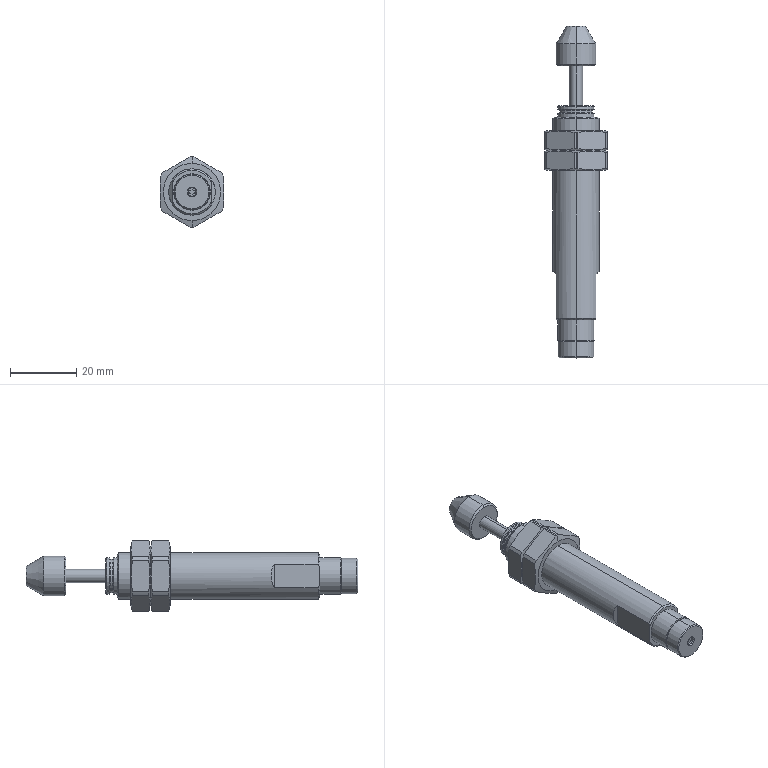Part | STEP file | Hydraulic buffer ACJ-1412 | 3 solids | 116 faces | box 19 x 100 x 21.289 mm | volume 13894 mm3 | plane 37 | cylinder 36 | cone 35 | torus 8 | commonest cylinder face diameters 21.289 x14 11 x6 13.188 x4 2.459 x2 4 x2 10 x2